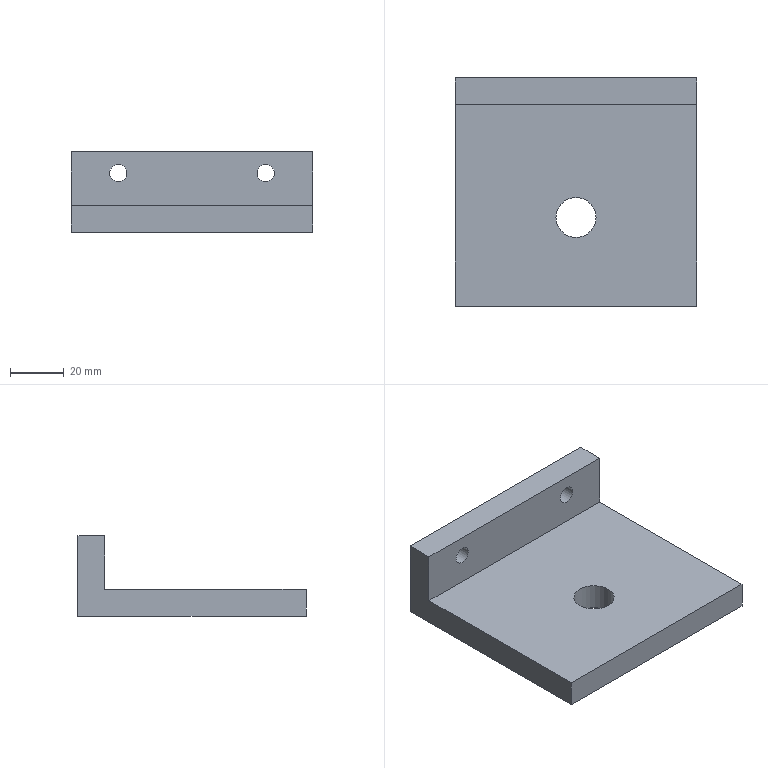Part | NX | 1 solid | 11 faces | box 90 x 85 x 30 mm | volume 92069 mm3 | plane 8 | cylinder 3 | commonest cylinder face diameters 6.5 x2 15 x1
STEP:
#1=CARTESIAN_POINT('',(45.,-37.5,0.));
#2=VERTEX_POINT('',#1);
#3=CARTESIAN_POINT('',(45.,47.5,0.));
#4=VERTEX_POINT('',#3);
#5=CARTESIAN_POINT('',(45.,37.5,0.));
#6=DIRECTION('',(0.,1.,0.));
#7=VECTOR('',#6,1000.);
#8=LINE('',#5,#7);
#9=EDGE_CURVE('',#2,#4,#8,.T.);
#10=ORIENTED_EDGE('',*,*,#9,.T.);
#11=CARTESIAN_POINT('',(45.,47.5,30.));
#12=VERTEX_POINT('',#11);
#13=CARTESIAN_POINT('',(45.,47.5,30.));
#14=DIRECTION('',(0.,0.,-1.));
#15=VECTOR('',#14,1000.);
#16=LINE('',#13,#15);
#17=EDGE_CURVE('',#12,#4,#16,.T.);
#18=ORIENTED_EDGE('',*,*,#17,.F.);
#19=CARTESIAN_POINT('',(45.,37.5,30.));
#20=VERTEX_POINT('',#19);
#21=CARTESIAN_POINT('',(45.,37.5,30.));
#22=DIRECTION('',(0.,1.,0.));
#23=VECTOR('',#22,1000.);
#24=LINE('',#21,#23);
#25=EDGE_CURVE('',#20,#12,#24,.T.);
#26=ORIENTED_EDGE('',*,*,#25,.F.);
#27=CARTESIAN_POINT('',(45.,37.5,10.));
#28=VERTEX_POINT('',#27);
#29=CARTESIAN_POINT('',(45.,37.5,30.));
#30=DIRECTION('',(0.,0.,-1.));
#31=VECTOR('',#30,1000.);
#32=LINE('',#29,#31);
#33=EDGE_CURVE('',#20,#28,#32,.T.);
#34=ORIENTED_EDGE('',*,*,#33,.T.);
#35=CARTESIAN_POINT('',(45.,-37.5,10.));
#36=VERTEX_POINT('',#35);
#37=CARTESIAN_POINT('',(45.,37.5,10.));
#38=DIRECTION('',(0.,1.,0.));
#39=VECTOR('',#38,1000.);
#40=LINE('',#37,#39);
#41=EDGE_CURVE('',#36,#28,#40,.T.);
#42=ORIENTED_EDGE('',*,*,#41,.F.);
#43=CARTESIAN_POINT('',(45.,-37.5,10.));
#44=DIRECTION('',(0.,0.,-1.));
#45=VECTOR('',#44,1000.);
#46=LINE('',#43,#45);
#47=EDGE_CURVE('',#36,#2,#46,.T.);
#48=ORIENTED_EDGE('',*,*,#47,.T.);
#49=EDGE_LOOP('',(#10,#18,#26,#34,#42,#48));
#50=FACE_BOUND('',#49,.T.);
#51=CARTESIAN_POINT('',(45.,37.5,10.));
#52=DIRECTION('',(-1.,0.,0.));
#53=DIRECTION('',(0.,-1.,0.));
#54=AXIS2_PLACEMENT_3D('',#51,#52,#53);
#55=PLANE('',#54);
#56=ADVANCED_FACE('',(#50),#55,.F.);
#57=CARTESIAN_POINT('',(-45.,47.5,0.));
#58=VERTEX_POINT('',#57);
#59=CARTESIAN_POINT('',(-45.,-37.5,0.));
#60=VERTEX_POINT('',#59);
#61=CARTESIAN_POINT('',(-45.,37.5,0.));
#62=DIRECTION('',(0.,-1.,0.));
#63=VECTOR('',#62,1000.);
#64=LINE('',#61,#63);
#65=EDGE_CURVE('',#58,#60,#64,.T.);
#66=ORIENTED_EDGE('',*,*,#65,.T.);
#67=CARTESIAN_POINT('',(-45.,-37.5,10.));
#68=VERTEX_POINT('',#67);
#69=CARTESIAN_POINT('',(-45.,-37.5,10.));
#70=DIRECTION('',(0.,0.,-1.));
#71=VECTOR('',#70,1000.);
#72=LINE('',#69,#71);
#73=EDGE_CURVE('',#68,#60,#72,.T.);
#74=ORIENTED_EDGE('',*,*,#73,.F.);
#75=CARTESIAN_POINT('',(-45.,37.5,10.));
#76=VERTEX_POINT('',#75);
#77=CARTESIAN_POINT('',(-45.,37.5,10.));
#78=DIRECTION('',(0.,-1.,0.));
#79=VECTOR('',#78,1000.);
#80=LINE('',#77,#79);
#81=EDGE_CURVE('',#76,#68,#80,.T.);
#82=ORIENTED_EDGE('',*,*,#81,.F.);
#83=CARTESIAN_POINT('',(-45.,37.5,30.));
#84=VERTEX_POINT('',#83);
#85=CARTESIAN_POINT('',(-45.,37.5,30.));
#86=DIRECTION('',(0.,0.,-1.));
#87=VECTOR('',#86,1000.);
#88=LINE('',#85,#87);
#89=EDGE_CURVE('',#84,#76,#88,.T.);
#90=ORIENTED_EDGE('',*,*,#89,.F.);
#91=CARTESIAN_POINT('',(-45.,47.5,30.));
#92=VERTEX_POINT('',#91);
#93=CARTESIAN_POINT('',(-45.,37.5,30.));
#94=DIRECTION('',(0.,-1.,0.));
#95=VECTOR('',#94,1000.);
#96=LINE('',#93,#95);
#97=EDGE_CURVE('',#92,#84,#96,.T.);
#98=ORIENTED_EDGE('',*,*,#97,.F.);
#99=CARTESIAN_POINT('',(-45.,47.5,30.));
#100=DIRECTION('',(0.,0.,-1.));
#101=VECTOR('',#100,1000.);
#102=LINE('',#99,#101);
#103=EDGE_CURVE('',#92,#58,#102,.T.);
#104=ORIENTED_EDGE('',*,*,#103,.T.);
#105=EDGE_LOOP('',(#66,#74,#82,#90,#98,#104));
#106=FACE_BOUND('',#105,.T.);
#107=CARTESIAN_POINT('',(-45.,37.5,10.));
#108=DIRECTION('',(1.,0.,0.));
#109=DIRECTION('',(0.,0.,-1.));
#110=AXIS2_PLACEMENT_3D('',#107,#108,#109);
#111=PLANE('',#110);
#112=ADVANCED_FACE('',(#106),#111,.F.);
#113=CARTESIAN_POINT('',(-45.,-37.5,0.));
#114=DIRECTION('',(1.,0.,0.));
#115=VECTOR('',#114,1000.);
#116=LINE('',#113,#115);
#117=EDGE_CURVE('',#60,#2,#116,.T.);
#118=ORIENTED_EDGE('',*,*,#117,.T.);
#119=ORIENTED_EDGE('',*,*,#47,.F.);
#120=CARTESIAN_POINT('',(-45.,-37.5,10.));
#121=DIRECTION('',(1.,0.,0.));
#122=VECTOR('',#121,1000.);
#123=LINE('',#120,#122);
#124=EDGE_CURVE('',#68,#36,#123,.T.);
#125=ORIENTED_EDGE('',*,*,#124,.F.);
#126=ORIENTED_EDGE('',*,*,#73,.T.);
#127=EDGE_LOOP('',(#118,#119,#125,#126));
#128=FACE_BOUND('',#127,.T.);
#129=CARTESIAN_POINT('',(-45.,-37.5,10.));
#130=DIRECTION('',(0.,1.,0.));
#131=DIRECTION('',(0.,0.,1.));
#132=AXIS2_PLACEMENT_3D('',#129,#130,#131);
#133=PLANE('',#132);
#134=ADVANCED_FACE('',(#128),#133,.F.);
#135=CARTESIAN_POINT('',(-45.,37.5,10.));
#136=DIRECTION('',(1.,0.,0.));
#137=VECTOR('',#136,1000.);
#138=LINE('',#135,#137);
#139=EDGE_CURVE('',#76,#28,#138,.T.);
#140=ORIENTED_EDGE('',*,*,#139,.F.);
#141=ORIENTED_EDGE('',*,*,#81,.T.);
#142=ORIENTED_EDGE('',*,*,#124,.T.);
#143=ORIENTED_EDGE('',*,*,#41,.T.);
#144=EDGE_LOOP('',(#140,#141,#142,#143));
#145=FACE_BOUND('',#144,.T.);
#146=CARTESIAN_POINT('',(7.5,-4.5,10.));
#147=VERTEX_POINT('',#146);
#148=CARTESIAN_POINT('',(0.,-4.5,10.));
#149=DIRECTION('',(0.,0.,1.));
#150=DIRECTION('',(1.,0.,0.));
#151=AXIS2_PLACEMENT_3D('',#148,#149,#150);
#152=CIRCLE('',#151,7.5);
#153=EDGE_CURVE('',#147,#147,#152,.T.);
#154=ORIENTED_EDGE('',*,*,#153,.F.);
#155=EDGE_LOOP('',(#154));
#156=FACE_BOUND('',#155,.T.);
#157=CARTESIAN_POINT('',(0.,0.,10.));
#158=DIRECTION('',(0.,0.,1.));
#159=DIRECTION('',(1.,0.,0.));
#160=AXIS2_PLACEMENT_3D('',#157,#158,#159);
#161=PLANE('',#160);
#162=ADVANCED_FACE('',(#145,#156),#161,.T.);
#163=CARTESIAN_POINT('',(7.5,-4.5,0.));
#164=VERTEX_POINT('',#163);
#165=CARTESIAN_POINT('',(0.,-4.5,0.));
#166=DIRECTION('',(0.,0.,1.));
#167=DIRECTION('',(1.,0.,0.));
#168=AXIS2_PLACEMENT_3D('',#165,#166,#167);
#169=CIRCLE('',#168,7.5);
#170=EDGE_CURVE('',#164,#164,#169,.T.);
#171=ORIENTED_EDGE('',*,*,#170,.T.);
#172=EDGE_LOOP('',(#171));
#173=FACE_BOUND('',#172,.T.);
#174=ORIENTED_EDGE('',*,*,#65,.F.);
#175=CARTESIAN_POINT('',(-50.,47.5,0.));
#176=DIRECTION('',(1.,0.,0.));
#177=VECTOR('',#176,1000.);
#178=LINE('',#175,#177);
#179=EDGE_CURVE('',#58,#4,#178,.T.);
#180=ORIENTED_EDGE('',*,*,#179,.T.);
#181=ORIENTED_EDGE('',*,*,#9,.F.);
#182=ORIENTED_EDGE('',*,*,#117,.F.);
#183=EDGE_LOOP('',(#174,#180,#181,#182));
#184=FACE_BOUND('',#183,.T.);
#185=CARTESIAN_POINT('',(0.,0.,0.));
#186=DIRECTION('',(0.,0.,1.));
#187=DIRECTION('',(1.,0.,0.));
#188=AXIS2_PLACEMENT_3D('',#185,#186,#187);
#189=PLANE('',#188);
#190=ADVANCED_FACE('',(#173,#184),#189,.F.);
#191=ORIENTED_EDGE('',*,*,#170,.F.);
#192=EDGE_LOOP('',(#191));
#193=FACE_BOUND('',#192,.T.);
#194=ORIENTED_EDGE('',*,*,#153,.T.);
#195=EDGE_LOOP('',(#194));
#196=FACE_BOUND('',#195,.T.);
#197=CARTESIAN_POINT('',(0.,-4.5,0.));
#198=DIRECTION('',(0.,0.,1.));
#199=DIRECTION('',(1.,0.,0.));
#200=AXIS2_PLACEMENT_3D('',#197,#198,#199);
#201=CYLINDRICAL_SURFACE('',#200,7.5);
#202=ADVANCED_FACE('',(#193,#196),#201,.F.);
#203=CARTESIAN_POINT('',(27.5,47.5,18.75));
#204=VERTEX_POINT('',#203);
#205=CARTESIAN_POINT('',(27.5,47.5,22.));
#206=DIRECTION('',(0.,-1.,0.));
#207=DIRECTION('',(0.,0.,-1.));
#208=AXIS2_PLACEMENT_3D('',#205,#206,#207);
#209=CIRCLE('',#208,3.25);
#210=EDGE_CURVE('',#204,#204,#209,.T.);
#211=ORIENTED_EDGE('',*,*,#210,.T.);
#212=EDGE_LOOP('',(#211));
#213=FACE_BOUND('',#212,.T.);
#214=CARTESIAN_POINT('',(-27.5,47.5,18.75));
#215=VERTEX_POINT('',#214);
#216=CARTESIAN_POINT('',(-27.5,47.5,22.));
#217=DIRECTION('',(0.,-1.,0.));
#218=DIRECTION('',(0.,0.,-1.));
#219=AXIS2_PLACEMENT_3D('',#216,#217,#218);
#220=CIRCLE('',#219,3.25);
#221=EDGE_CURVE('',#215,#215,#220,.T.);
#222=ORIENTED_EDGE('',*,*,#221,.T.);
#223=EDGE_LOOP('',(#222));
#224=FACE_BOUND('',#223,.T.);
#225=ORIENTED_EDGE('',*,*,#179,.F.);
#226=ORIENTED_EDGE('',*,*,#103,.F.);
#227=CARTESIAN_POINT('',(-45.,47.5,30.));
#228=DIRECTION('',(-1.,0.,0.));
#229=VECTOR('',#228,1000.);
#230=LINE('',#227,#229);
#231=EDGE_CURVE('',#12,#92,#230,.T.);
#232=ORIENTED_EDGE('',*,*,#231,.F.);
#233=ORIENTED_EDGE('',*,*,#17,.T.);
#234=EDGE_LOOP('',(#225,#226,#232,#233));
#235=FACE_BOUND('',#234,.T.);
#236=CARTESIAN_POINT('',(0.,47.5,0.));
#237=DIRECTION('',(0.,-1.,0.));
#238=DIRECTION('',(0.,0.,-1.));
#239=AXIS2_PLACEMENT_3D('',#236,#237,#238);
#240=PLANE('',#239);
#241=ADVANCED_FACE('',(#213,#224,#235),#240,.F.);
#242=CARTESIAN_POINT('',(27.5,37.5,18.75));
#243=VERTEX_POINT('',#242);
#244=CARTESIAN_POINT('',(27.5,37.5,22.));
#245=DIRECTION('',(0.,-1.,0.));
#246=DIRECTION('',(0.,0.,-1.));
#247=AXIS2_PLACEMENT_3D('',#244,#245,#246);
#248=CIRCLE('',#247,3.25);
#249=EDGE_CURVE('',#243,#243,#248,.T.);
#250=ORIENTED_EDGE('',*,*,#249,.F.);
#251=EDGE_LOOP('',(#250));
#252=FACE_BOUND('',#251,.T.);
#253=CARTESIAN_POINT('',(-27.5,37.5,18.75));
#254=VERTEX_POINT('',#253);
#255=CARTESIAN_POINT('',(-27.5,37.5,22.));
#256=DIRECTION('',(0.,-1.,0.));
#257=DIRECTION('',(0.,0.,-1.));
#258=AXIS2_PLACEMENT_3D('',#255,#256,#257);
#259=CIRCLE('',#258,3.25);
#260=EDGE_CURVE('',#254,#254,#259,.T.);
#261=ORIENTED_EDGE('',*,*,#260,.F.);
#262=EDGE_LOOP('',(#261));
#263=FACE_BOUND('',#262,.T.);
#264=ORIENTED_EDGE('',*,*,#139,.T.);
#265=ORIENTED_EDGE('',*,*,#33,.F.);
#266=CARTESIAN_POINT('',(-45.,37.5,30.));
#267=DIRECTION('',(1.,0.,0.));
#268=VECTOR('',#267,1000.);
#269=LINE('',#266,#268);
#270=EDGE_CURVE('',#84,#20,#269,.T.);
#271=ORIENTED_EDGE('',*,*,#270,.F.);
#272=ORIENTED_EDGE('',*,*,#89,.T.);
#273=EDGE_LOOP('',(#264,#265,#271,#272));
#274=FACE_BOUND('',#273,.T.);
#275=CARTESIAN_POINT('',(-45.,37.5,30.));
#276=DIRECTION('',(0.,1.,0.));
#277=DIRECTION('',(0.,0.,1.));
#278=AXIS2_PLACEMENT_3D('',#275,#276,#277);
#279=PLANE('',#278);
#280=ADVANCED_FACE('',(#252,#263,#274),#279,.F.);
#281=ORIENTED_EDGE('',*,*,#97,.T.);
#282=ORIENTED_EDGE('',*,*,#270,.T.);
#283=ORIENTED_EDGE('',*,*,#25,.T.);
#284=ORIENTED_EDGE('',*,*,#231,.T.);
#285=EDGE_LOOP('',(#281,#282,#283,#284));
#286=FACE_BOUND('',#285,.T.);
#287=CARTESIAN_POINT('',(0.,0.,30.));
#288=DIRECTION('',(0.,0.,-1.));
#289=DIRECTION('',(-1.,0.,0.));
#290=AXIS2_PLACEMENT_3D('',#287,#288,#289);
#291=PLANE('',#290);
#292=ADVANCED_FACE('',(#286),#291,.F.);
#293=ORIENTED_EDGE('',*,*,#221,.F.);
#294=EDGE_LOOP('',(#293));
#295=FACE_BOUND('',#294,.T.);
#296=ORIENTED_EDGE('',*,*,#260,.T.);
#297=EDGE_LOOP('',(#296));
#298=FACE_BOUND('',#297,.T.);
#299=CARTESIAN_POINT('',(-27.5,37.5,22.));
#300=DIRECTION('',(0.,-1.,0.));
#301=DIRECTION('',(0.,0.,-1.));
#302=AXIS2_PLACEMENT_3D('',#299,#300,#301);
#303=CYLINDRICAL_SURFACE('',#302,3.25);
#304=ADVANCED_FACE('',(#295,#298),#303,.F.);
#305=ORIENTED_EDGE('',*,*,#210,.F.);
#306=EDGE_LOOP('',(#305));
#307=FACE_BOUND('',#306,.T.);
#308=ORIENTED_EDGE('',*,*,#249,.T.);
#309=EDGE_LOOP('',(#308));
#310=FACE_BOUND('',#309,.T.);
#311=CARTESIAN_POINT('',(27.5,37.5,22.));
#312=DIRECTION('',(0.,-1.,0.));
#313=DIRECTION('',(0.,0.,-1.));
#314=AXIS2_PLACEMENT_3D('',#311,#312,#313);
#315=CYLINDRICAL_SURFACE('',#314,3.25);
#316=ADVANCED_FACE('',(#307,#310),#315,.F.);
#317=CLOSED_SHELL('',(#56,#112,#134,#162,#190,#202,#241,#280,#292,#304,#316));
#318=MANIFOLD_SOLID_BREP('',#317);
#319=(LENGTH_UNIT()NAMED_UNIT(*)SI_UNIT(.MILLI.,.METRE.));
#320=UNCERTAINTY_MEASURE_WITH_UNIT(LENGTH_MEASURE(0.00001),#319,'','');
#321=(NAMED_UNIT(*)PLANE_ANGLE_UNIT()SI_UNIT($,.RADIAN.));
#322=(NAMED_UNIT(*)SI_UNIT($,.STERADIAN.)SOLID_ANGLE_UNIT());
#323=(GEOMETRIC_REPRESENTATION_CONTEXT(3)GLOBAL_UNCERTAINTY_ASSIGNED_CONTEXT((#320))GLOBAL_UNIT_ASSIGNED_CONTEXT((#319,#321,#322))REPRESENTATION_CONTEXT('',''));
#324=ADVANCED_BREP_SHAPE_REPRESENTATION('',(#318),#323);